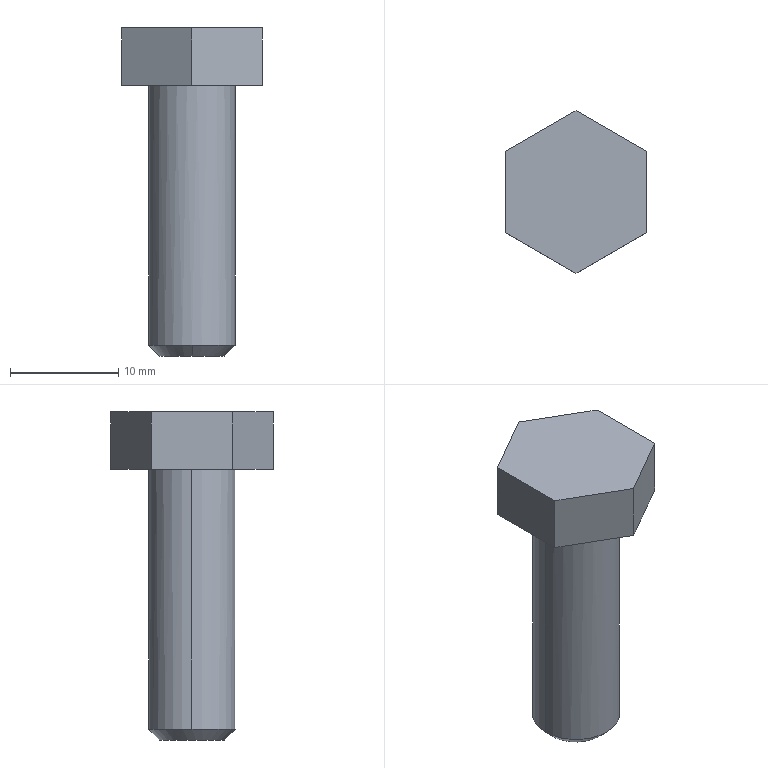Part | STEP file | 921281610 | 1 solid | 13 faces | box 13 x 15.011 x 30.3 mm | volume 2021 mm3 | plane 9 | cylinder 2 | cone 2 | commonest cylinder face diameters 8 x2
STEP:
#1=CARTESIAN_POINT('',(0.,4.,-24.));
#2=VERTEX_POINT('',#1);
#3=CARTESIAN_POINT('',(-4.,0.,-24.));
#4=VERTEX_POINT('',#3);
#5=CARTESIAN_POINT('',(0.,0.,-24.));
#6=DIRECTION('',(0.,0.,1.));
#7=DIRECTION('',(1.,0.,0.));
#8=AXIS2_PLACEMENT_3D('',#5,#6,#7);
#9=CIRCLE('',#8,4.);
#10=EDGE_CURVE('',#2,#4,#9,.T.);
#11=ORIENTED_EDGE('',*,*,#10,.T.);
#12=CARTESIAN_POINT('',(-4.,0.,0.));
#13=VERTEX_POINT('',#12);
#14=CARTESIAN_POINT('',(-4.,0.,-25.));
#15=DIRECTION('',(0.,0.,1.));
#16=VECTOR('',#15,1000.);
#17=LINE('',#14,#16);
#18=EDGE_CURVE('',#4,#13,#17,.T.);
#19=ORIENTED_EDGE('',*,*,#18,.T.);
#20=CARTESIAN_POINT('',(4.,0.,0.));
#21=VERTEX_POINT('',#20);
#22=CARTESIAN_POINT('',(0.,0.,0.));
#23=DIRECTION('',(0.,0.,-1.));
#24=DIRECTION('',(1.,0.,0.));
#25=AXIS2_PLACEMENT_3D('',#22,#23,#24);
#26=CIRCLE('',#25,4.);
#27=EDGE_CURVE('',#13,#21,#26,.T.);
#28=ORIENTED_EDGE('',*,*,#27,.T.);
#29=CARTESIAN_POINT('',(4.,0.,-24.));
#30=VERTEX_POINT('',#29);
#31=CARTESIAN_POINT('',(4.,0.,-25.));
#32=DIRECTION('',(0.,0.,1.));
#33=VECTOR('',#32,1000.);
#34=LINE('',#31,#33);
#35=EDGE_CURVE('',#30,#21,#34,.T.);
#36=ORIENTED_EDGE('',*,*,#35,.F.);
#37=CARTESIAN_POINT('',(0.,0.,-24.));
#38=DIRECTION('',(0.,0.,1.));
#39=DIRECTION('',(1.,0.,0.));
#40=AXIS2_PLACEMENT_3D('',#37,#38,#39);
#41=CIRCLE('',#40,4.);
#42=EDGE_CURVE('',#30,#2,#41,.T.);
#43=ORIENTED_EDGE('',*,*,#42,.T.);
#44=EDGE_LOOP('',(#11,#19,#28,#36,#43));
#45=FACE_OUTER_BOUND('',#44,.T.);
#46=CARTESIAN_POINT('',(0.,0.,-25.));
#47=DIRECTION('',(0.,0.,1.));
#48=DIRECTION('',(1.,0.,0.));
#49=AXIS2_PLACEMENT_3D('',#46,#47,#48);
#50=CYLINDRICAL_SURFACE('',#49,4.);
#51=ADVANCED_FACE('',(#45),#50,.T.);
#52=CARTESIAN_POINT('',(0.,-3.,-25.));
#53=VERTEX_POINT('',#52);
#54=CARTESIAN_POINT('',(0.,3.,-25.));
#55=VERTEX_POINT('',#54);
#56=CARTESIAN_POINT('',(0.,0.,-25.));
#57=DIRECTION('',(0.,0.,1.));
#58=DIRECTION('',(0.,-1.,0.));
#59=AXIS2_PLACEMENT_3D('',#56,#57,#58);
#60=CIRCLE('',#59,3.);
#61=EDGE_CURVE('',#53,#55,#60,.T.);
#62=ORIENTED_EDGE('',*,*,#61,.T.);
#63=CARTESIAN_POINT('',(0.,4.,-24.));
#64=DIRECTION('',(0.,0.7071,0.7071));
#65=VECTOR('',#64,1000.);
#66=LINE('',#63,#65);
#67=EDGE_CURVE('',#55,#2,#66,.T.);
#68=ORIENTED_EDGE('',*,*,#67,.T.);
#69=ORIENTED_EDGE('',*,*,#42,.F.);
#70=CARTESIAN_POINT('',(0.,-4.,-24.));
#71=VERTEX_POINT('',#70);
#72=CARTESIAN_POINT('',(0.,0.,-24.));
#73=DIRECTION('',(0.,0.,1.));
#74=DIRECTION('',(1.,0.,0.));
#75=AXIS2_PLACEMENT_3D('',#72,#73,#74);
#76=CIRCLE('',#75,4.);
#77=EDGE_CURVE('',#71,#30,#76,.T.);
#78=ORIENTED_EDGE('',*,*,#77,.F.);
#79=CARTESIAN_POINT('',(0.,-4.,-24.));
#80=DIRECTION('',(0.,-0.7071,0.7071));
#81=VECTOR('',#80,1000.);
#82=LINE('',#79,#81);
#83=EDGE_CURVE('',#53,#71,#82,.T.);
#84=ORIENTED_EDGE('',*,*,#83,.F.);
#85=EDGE_LOOP('',(#62,#68,#69,#78,#84));
#86=FACE_OUTER_BOUND('',#85,.T.);
#87=CARTESIAN_POINT('',(0.,0.,-24.));
#88=DIRECTION('',(0.,0.,1.));
#89=DIRECTION('',(0.,-1.,0.));
#90=AXIS2_PLACEMENT_3D('',#87,#88,#89);
#91=CONICAL_SURFACE('',#90,4.,0.7854);
#92=ADVANCED_FACE('',(#86),#91,.T.);
#93=ORIENTED_EDGE('',*,*,#18,.F.);
#94=CARTESIAN_POINT('',(0.,0.,-24.));
#95=DIRECTION('',(0.,0.,1.));
#96=DIRECTION('',(1.,0.,0.));
#97=AXIS2_PLACEMENT_3D('',#94,#95,#96);
#98=CIRCLE('',#97,4.);
#99=EDGE_CURVE('',#4,#71,#98,.T.);
#100=ORIENTED_EDGE('',*,*,#99,.T.);
#101=ORIENTED_EDGE('',*,*,#77,.T.);
#102=ORIENTED_EDGE('',*,*,#35,.T.);
#103=CARTESIAN_POINT('',(0.,0.,0.));
#104=DIRECTION('',(0.,0.,-1.));
#105=DIRECTION('',(1.,0.,0.));
#106=AXIS2_PLACEMENT_3D('',#103,#104,#105);
#107=CIRCLE('',#106,4.);
#108=EDGE_CURVE('',#21,#13,#107,.T.);
#109=ORIENTED_EDGE('',*,*,#108,.T.);
#110=EDGE_LOOP('',(#93,#100,#101,#102,#109));
#111=FACE_OUTER_BOUND('',#110,.T.);
#112=CARTESIAN_POINT('',(0.,0.,-25.));
#113=DIRECTION('',(0.,0.,1.));
#114=DIRECTION('',(1.,0.,0.));
#115=AXIS2_PLACEMENT_3D('',#112,#113,#114);
#116=CYLINDRICAL_SURFACE('',#115,4.);
#117=ADVANCED_FACE('',(#111),#116,.T.);
#118=ORIENTED_EDGE('',*,*,#108,.F.);
#119=ORIENTED_EDGE('',*,*,#27,.F.);
#120=EDGE_LOOP('',(#118,#119));
#121=FACE_BOUND('',#120,.T.);
#122=CARTESIAN_POINT('',(-6.5,-3.753,0.));
#123=VERTEX_POINT('',#122);
#124=CARTESIAN_POINT('',(0.,-7.506,0.));
#125=VERTEX_POINT('',#124);
#126=CARTESIAN_POINT('',(-6.5,-3.753,0.));
#127=DIRECTION('',(0.866,-0.5,0.));
#128=VECTOR('',#127,1000.);
#129=LINE('',#126,#128);
#130=EDGE_CURVE('',#123,#125,#129,.T.);
#131=ORIENTED_EDGE('',*,*,#130,.F.);
#132=CARTESIAN_POINT('',(-6.5,3.753,0.));
#133=VERTEX_POINT('',#132);
#134=CARTESIAN_POINT('',(-6.5,0.,0.));
#135=DIRECTION('',(0.,-1.,0.));
#136=VECTOR('',#135,1000.);
#137=LINE('',#134,#136);
#138=EDGE_CURVE('',#133,#123,#137,.T.);
#139=ORIENTED_EDGE('',*,*,#138,.F.);
#140=CARTESIAN_POINT('',(0.,7.506,0.));
#141=VERTEX_POINT('',#140);
#142=CARTESIAN_POINT('',(0.,7.506,0.));
#143=DIRECTION('',(-0.866,-0.5,0.));
#144=VECTOR('',#143,1000.);
#145=LINE('',#142,#144);
#146=EDGE_CURVE('',#141,#133,#145,.T.);
#147=ORIENTED_EDGE('',*,*,#146,.F.);
#148=CARTESIAN_POINT('',(6.5,3.753,0.));
#149=VERTEX_POINT('',#148);
#150=CARTESIAN_POINT('',(6.5,3.753,0.));
#151=DIRECTION('',(-0.866,0.5,0.));
#152=VECTOR('',#151,1000.);
#153=LINE('',#150,#152);
#154=EDGE_CURVE('',#149,#141,#153,.T.);
#155=ORIENTED_EDGE('',*,*,#154,.F.);
#156=CARTESIAN_POINT('',(6.5,-3.753,0.));
#157=VERTEX_POINT('',#156);
#158=CARTESIAN_POINT('',(6.5,0.,0.));
#159=DIRECTION('',(0.,1.,0.));
#160=VECTOR('',#159,1000.);
#161=LINE('',#158,#160);
#162=EDGE_CURVE('',#157,#149,#161,.T.);
#163=ORIENTED_EDGE('',*,*,#162,.F.);
#164=CARTESIAN_POINT('',(0.,-7.506,0.));
#165=DIRECTION('',(0.866,0.5,0.));
#166=VECTOR('',#165,1000.);
#167=LINE('',#164,#166);
#168=EDGE_CURVE('',#125,#157,#167,.T.);
#169=ORIENTED_EDGE('',*,*,#168,.F.);
#170=EDGE_LOOP('',(#131,#139,#147,#155,#163,#169));
#171=FACE_OUTER_BOUND('',#170,.T.);
#172=CARTESIAN_POINT('',(0.,0.,0.));
#173=DIRECTION('',(0.,0.,1.));
#174=DIRECTION('',(1.,0.,0.));
#175=AXIS2_PLACEMENT_3D('',#172,#173,#174);
#176=PLANE('',#175);
#177=ADVANCED_FACE('',(#121,#171),#176,.F.);
#178=ORIENTED_EDGE('',*,*,#67,.F.);
#179=CARTESIAN_POINT('',(0.,0.,-25.));
#180=DIRECTION('',(0.,0.,1.));
#181=DIRECTION('',(0.,-1.,0.));
#182=AXIS2_PLACEMENT_3D('',#179,#180,#181);
#183=CIRCLE('',#182,3.);
#184=EDGE_CURVE('',#55,#53,#183,.T.);
#185=ORIENTED_EDGE('',*,*,#184,.T.);
#186=ORIENTED_EDGE('',*,*,#83,.T.);
#187=ORIENTED_EDGE('',*,*,#99,.F.);
#188=ORIENTED_EDGE('',*,*,#10,.F.);
#189=EDGE_LOOP('',(#178,#185,#186,#187,#188));
#190=FACE_OUTER_BOUND('',#189,.T.);
#191=CARTESIAN_POINT('',(0.,0.,-24.));
#192=DIRECTION('',(0.,0.,1.));
#193=DIRECTION('',(0.,-1.,0.));
#194=AXIS2_PLACEMENT_3D('',#191,#192,#193);
#195=CONICAL_SURFACE('',#194,4.,0.7854);
#196=ADVANCED_FACE('',(#190),#195,.T.);
#197=CARTESIAN_POINT('',(6.5,-3.753,5.3));
#198=VERTEX_POINT('',#197);
#199=CARTESIAN_POINT('',(6.5,-3.753,5.3));
#200=DIRECTION('',(0.,0.,-1.));
#201=VECTOR('',#200,1000.);
#202=LINE('',#199,#201);
#203=EDGE_CURVE('',#198,#157,#202,.T.);
#204=ORIENTED_EDGE('',*,*,#203,.F.);
#205=CARTESIAN_POINT('',(0.,-7.506,5.3));
#206=VERTEX_POINT('',#205);
#207=CARTESIAN_POINT('',(0.,-7.506,5.3));
#208=DIRECTION('',(0.866,0.5,0.));
#209=VECTOR('',#208,1000.);
#210=LINE('',#207,#209);
#211=EDGE_CURVE('',#206,#198,#210,.T.);
#212=ORIENTED_EDGE('',*,*,#211,.F.);
#213=CARTESIAN_POINT('',(0.,-7.506,5.3));
#214=DIRECTION('',(0.,0.,1.));
#215=VECTOR('',#214,1000.);
#216=LINE('',#213,#215);
#217=EDGE_CURVE('',#125,#206,#216,.T.);
#218=ORIENTED_EDGE('',*,*,#217,.F.);
#219=ORIENTED_EDGE('',*,*,#168,.T.);
#220=EDGE_LOOP('',(#204,#212,#218,#219));
#221=FACE_OUTER_BOUND('',#220,.T.);
#222=CARTESIAN_POINT('',(0.,-7.506,5.3));
#223=DIRECTION('',(-0.5,0.866,0.));
#224=DIRECTION('',(-0.866,-0.5,0.));
#225=AXIS2_PLACEMENT_3D('',#222,#223,#224);
#226=PLANE('',#225);
#227=ADVANCED_FACE('',(#221),#226,.F.);
#228=ORIENTED_EDGE('',*,*,#217,.T.);
#229=CARTESIAN_POINT('',(-6.5,-3.753,5.3));
#230=VERTEX_POINT('',#229);
#231=CARTESIAN_POINT('',(-6.5,-3.753,5.3));
#232=DIRECTION('',(0.866,-0.5,0.));
#233=VECTOR('',#232,1000.);
#234=LINE('',#231,#233);
#235=EDGE_CURVE('',#230,#206,#234,.T.);
#236=ORIENTED_EDGE('',*,*,#235,.F.);
#237=CARTESIAN_POINT('',(-6.5,-3.753,5.3));
#238=DIRECTION('',(0.,0.,1.));
#239=VECTOR('',#238,1000.);
#240=LINE('',#237,#239);
#241=EDGE_CURVE('',#123,#230,#240,.T.);
#242=ORIENTED_EDGE('',*,*,#241,.F.);
#243=ORIENTED_EDGE('',*,*,#130,.T.);
#244=EDGE_LOOP('',(#228,#236,#242,#243));
#245=FACE_OUTER_BOUND('',#244,.T.);
#246=CARTESIAN_POINT('',(-6.5,-3.753,5.3));
#247=DIRECTION('',(0.5,0.866,0.));
#248=DIRECTION('',(-0.866,0.5,0.));
#249=AXIS2_PLACEMENT_3D('',#246,#247,#248);
#250=PLANE('',#249);
#251=ADVANCED_FACE('',(#245),#250,.F.);
#252=ORIENTED_EDGE('',*,*,#241,.T.);
#253=CARTESIAN_POINT('',(-6.5,3.753,5.3));
#254=VERTEX_POINT('',#253);
#255=CARTESIAN_POINT('',(-6.5,3.753,5.3));
#256=DIRECTION('',(0.,-1.,0.));
#257=VECTOR('',#256,1000.);
#258=LINE('',#255,#257);
#259=EDGE_CURVE('',#254,#230,#258,.T.);
#260=ORIENTED_EDGE('',*,*,#259,.F.);
#261=CARTESIAN_POINT('',(-6.5,3.753,5.3));
#262=DIRECTION('',(0.,0.,1.));
#263=VECTOR('',#262,1000.);
#264=LINE('',#261,#263);
#265=EDGE_CURVE('',#133,#254,#264,.T.);
#266=ORIENTED_EDGE('',*,*,#265,.F.);
#267=ORIENTED_EDGE('',*,*,#138,.T.);
#268=EDGE_LOOP('',(#252,#260,#266,#267));
#269=FACE_OUTER_BOUND('',#268,.T.);
#270=CARTESIAN_POINT('',(-6.5,3.753,5.3));
#271=DIRECTION('',(1.,0.,0.));
#272=DIRECTION('',(0.,0.,-1.));
#273=AXIS2_PLACEMENT_3D('',#270,#271,#272);
#274=PLANE('',#273);
#275=ADVANCED_FACE('',(#269),#274,.F.);
#276=ORIENTED_EDGE('',*,*,#265,.T.);
#277=CARTESIAN_POINT('',(0.,7.506,5.3));
#278=VERTEX_POINT('',#277);
#279=CARTESIAN_POINT('',(0.,7.506,5.3));
#280=DIRECTION('',(-0.866,-0.5,0.));
#281=VECTOR('',#280,1000.);
#282=LINE('',#279,#281);
#283=EDGE_CURVE('',#278,#254,#282,.T.);
#284=ORIENTED_EDGE('',*,*,#283,.F.);
#285=CARTESIAN_POINT('',(0.,7.506,5.3));
#286=DIRECTION('',(0.,0.,1.));
#287=VECTOR('',#286,1000.);
#288=LINE('',#285,#287);
#289=EDGE_CURVE('',#141,#278,#288,.T.);
#290=ORIENTED_EDGE('',*,*,#289,.F.);
#291=ORIENTED_EDGE('',*,*,#146,.T.);
#292=EDGE_LOOP('',(#276,#284,#290,#291));
#293=FACE_OUTER_BOUND('',#292,.T.);
#294=CARTESIAN_POINT('',(0.,7.506,5.3));
#295=DIRECTION('',(0.5,-0.866,0.));
#296=DIRECTION('',(0.866,0.5,0.));
#297=AXIS2_PLACEMENT_3D('',#294,#295,#296);
#298=PLANE('',#297);
#299=ADVANCED_FACE('',(#293),#298,.F.);
#300=ORIENTED_EDGE('',*,*,#289,.T.);
#301=CARTESIAN_POINT('',(6.5,3.753,5.3));
#302=VERTEX_POINT('',#301);
#303=CARTESIAN_POINT('',(6.5,3.753,5.3));
#304=DIRECTION('',(-0.866,0.5,0.));
#305=VECTOR('',#304,1000.);
#306=LINE('',#303,#305);
#307=EDGE_CURVE('',#302,#278,#306,.T.);
#308=ORIENTED_EDGE('',*,*,#307,.F.);
#309=CARTESIAN_POINT('',(6.5,3.753,5.3));
#310=DIRECTION('',(0.,0.,1.));
#311=VECTOR('',#310,1000.);
#312=LINE('',#309,#311);
#313=EDGE_CURVE('',#149,#302,#312,.T.);
#314=ORIENTED_EDGE('',*,*,#313,.F.);
#315=ORIENTED_EDGE('',*,*,#154,.T.);
#316=EDGE_LOOP('',(#300,#308,#314,#315));
#317=FACE_OUTER_BOUND('',#316,.T.);
#318=CARTESIAN_POINT('',(6.5,3.753,5.3));
#319=DIRECTION('',(-0.5,-0.866,0.));
#320=DIRECTION('',(0.866,-0.5,0.));
#321=AXIS2_PLACEMENT_3D('',#318,#319,#320);
#322=PLANE('',#321);
#323=ADVANCED_FACE('',(#317),#322,.F.);
#324=ORIENTED_EDGE('',*,*,#313,.T.);
#325=CARTESIAN_POINT('',(6.5,-3.753,5.3));
#326=DIRECTION('',(0.,1.,0.));
#327=VECTOR('',#326,1000.);
#328=LINE('',#325,#327);
#329=EDGE_CURVE('',#198,#302,#328,.T.);
#330=ORIENTED_EDGE('',*,*,#329,.F.);
#331=ORIENTED_EDGE('',*,*,#203,.T.);
#332=ORIENTED_EDGE('',*,*,#162,.T.);
#333=EDGE_LOOP('',(#324,#330,#331,#332));
#334=FACE_OUTER_BOUND('',#333,.T.);
#335=CARTESIAN_POINT('',(6.5,-3.753,5.3));
#336=DIRECTION('',(-1.,0.,0.));
#337=DIRECTION('',(0.,0.,1.));
#338=AXIS2_PLACEMENT_3D('',#335,#336,#337);
#339=PLANE('',#338);
#340=ADVANCED_FACE('',(#334),#339,.F.);
#341=ORIENTED_EDGE('',*,*,#61,.F.);
#342=ORIENTED_EDGE('',*,*,#184,.F.);
#343=EDGE_LOOP('',(#341,#342));
#344=FACE_OUTER_BOUND('',#343,.T.);
#345=CARTESIAN_POINT('',(0.,0.,-25.));
#346=DIRECTION('',(0.,0.,-1.));
#347=DIRECTION('',(-1.,0.,0.));
#348=AXIS2_PLACEMENT_3D('',#345,#346,#347);
#349=PLANE('',#348);
#350=ADVANCED_FACE('',(#344),#349,.T.);
#351=ORIENTED_EDGE('',*,*,#259,.T.);
#352=ORIENTED_EDGE('',*,*,#235,.T.);
#353=ORIENTED_EDGE('',*,*,#211,.T.);
#354=ORIENTED_EDGE('',*,*,#329,.T.);
#355=ORIENTED_EDGE('',*,*,#307,.T.);
#356=ORIENTED_EDGE('',*,*,#283,.T.);
#357=EDGE_LOOP('',(#351,#352,#353,#354,#355,#356));
#358=FACE_OUTER_BOUND('',#357,.T.);
#359=CARTESIAN_POINT('',(0.,0.,5.3));
#360=DIRECTION('',(0.,0.,1.));
#361=DIRECTION('',(1.,0.,0.));
#362=AXIS2_PLACEMENT_3D('',#359,#360,#361);
#363=PLANE('',#362);
#364=ADVANCED_FACE('',(#358),#363,.T.);
#365=CLOSED_SHELL('',(#51,#92,#117,#177,#196,#227,#251,#275,#299,#323,#340,#350,#364));
#366=MANIFOLD_SOLID_BREP('',#365);
#367=CARTESIAN_POINT('',(0.,0.,0.));
#368=DIRECTION('',(0.,0.,1.));
#369=DIRECTION('',(1.,0.,0.));
#370=AXIS2_PLACEMENT_3D('',#367,#368,#369);
#371=(LENGTH_UNIT()NAMED_UNIT(*)SI_UNIT(.MILLI.,.METRE.));
#372=UNCERTAINTY_MEASURE_WITH_UNIT(LENGTH_MEASURE(0.00001),#371,'','');
#373=(NAMED_UNIT(*)PLANE_ANGLE_UNIT()SI_UNIT($,.RADIAN.));
#374=(NAMED_UNIT(*)SI_UNIT($,.STERADIAN.)SOLID_ANGLE_UNIT());
#375=(GEOMETRIC_REPRESENTATION_CONTEXT(3)GLOBAL_UNCERTAINTY_ASSIGNED_CONTEXT((#372))GLOBAL_UNIT_ASSIGNED_CONTEXT((#371,#373,#374))REPRESENTATION_CONTEXT('',''));
#376=ADVANCED_BREP_SHAPE_REPRESENTATION('',(#366,#370),#375);